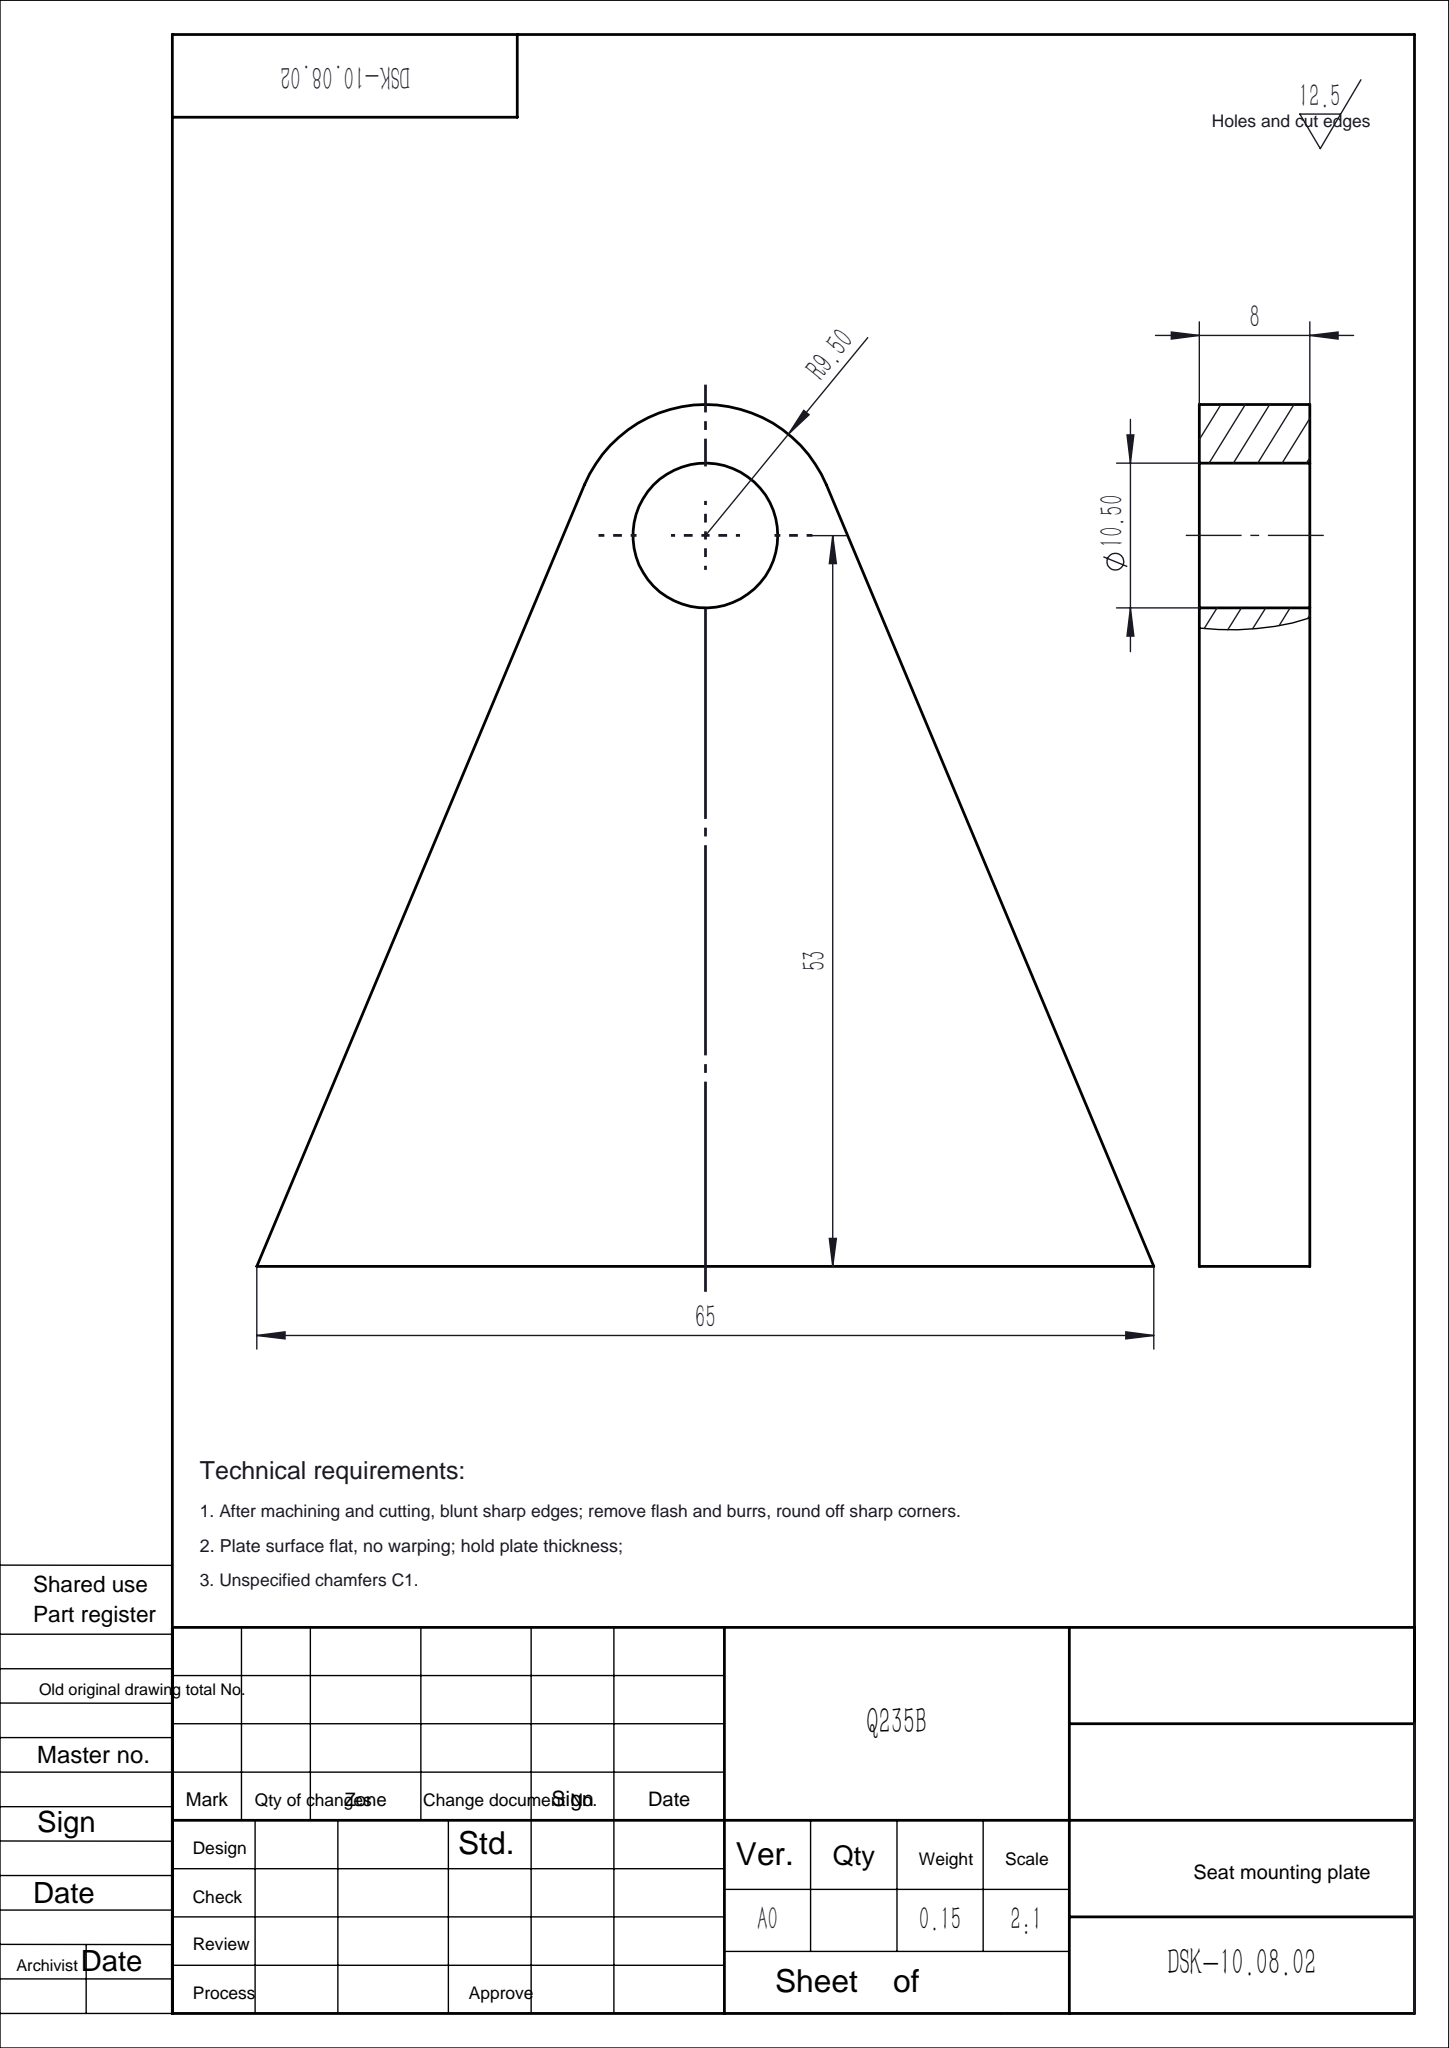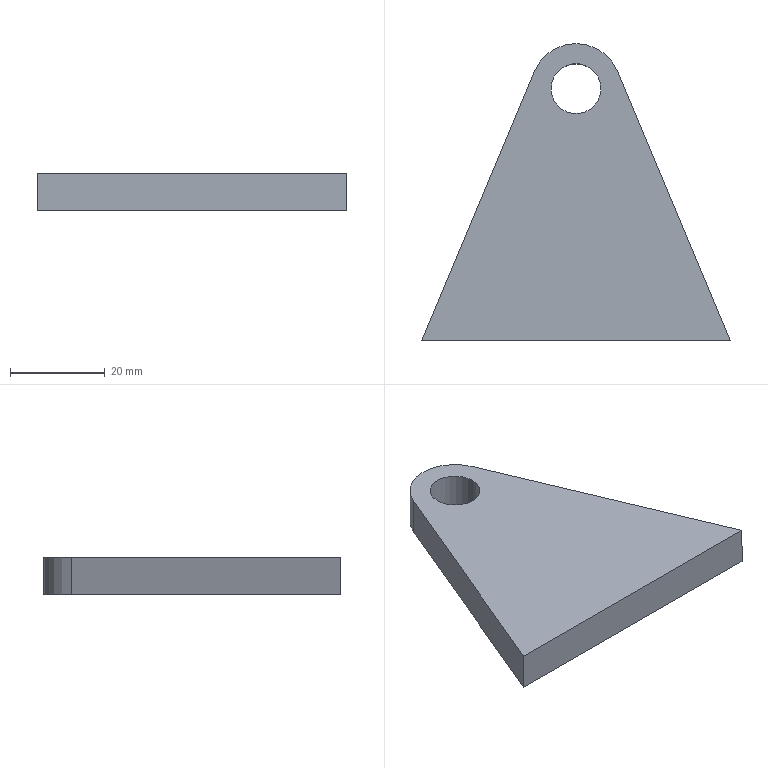Part | SolidWorks | features Extrusion 1 | 1 solid | 8 faces | box 65 x 62.5 x 8 mm | volume 18605 mm3 | plane 5 | cylinder 3 | commonest cylinder face diameters 10.5 x2 19 x1
STEP:
#1=CARTESIAN_POINT('',(-5.25,53.,8.));
#2=VERTEX_POINT('',#1);
#3=CARTESIAN_POINT('',(5.25,53.,8.));
#4=VERTEX_POINT('',#3);
#5=CARTESIAN_POINT('',(0.,53.,8.));
#6=DIRECTION('',(0.,0.,1.));
#7=DIRECTION('',(1.,0.,0.));
#8=AXIS2_PLACEMENT_3D('',#5,#6,#7);
#9=CIRCLE('',#8,5.25);
#10=EDGE_CURVE('',#2,#4,#9,.T.);
#11=ORIENTED_EDGE('',*,*,#10,.T.);
#12=CARTESIAN_POINT('',(5.25,53.,0.));
#13=VERTEX_POINT('',#12);
#14=CARTESIAN_POINT('',(5.25,53.,8.));
#15=DIRECTION('',(0.,0.,-1.));
#16=VECTOR('',#15,1000.);
#17=LINE('',#14,#16);
#18=EDGE_CURVE('',#4,#13,#17,.T.);
#19=ORIENTED_EDGE('',*,*,#18,.T.);
#20=CARTESIAN_POINT('',(-5.25,53.,0.));
#21=VERTEX_POINT('',#20);
#22=CARTESIAN_POINT('',(0.,53.,0.));
#23=DIRECTION('',(0.,0.,1.));
#24=DIRECTION('',(1.,0.,0.));
#25=AXIS2_PLACEMENT_3D('',#22,#23,#24);
#26=CIRCLE('',#25,5.25);
#27=EDGE_CURVE('',#21,#13,#26,.T.);
#28=ORIENTED_EDGE('',*,*,#27,.F.);
#29=CARTESIAN_POINT('',(-5.25,53.,8.));
#30=DIRECTION('',(0.,0.,-1.));
#31=VECTOR('',#30,1000.);
#32=LINE('',#29,#31);
#33=EDGE_CURVE('',#2,#21,#32,.T.);
#34=ORIENTED_EDGE('',*,*,#33,.F.);
#35=EDGE_LOOP('',(#11,#19,#28,#34));
#36=FACE_OUTER_BOUND('',#35,.T.);
#37=CARTESIAN_POINT('',(0.,53.,8.));
#38=DIRECTION('',(0.,0.,-1.));
#39=DIRECTION('',(-1.,0.,0.));
#40=AXIS2_PLACEMENT_3D('',#37,#38,#39);
#41=CYLINDRICAL_SURFACE('',#40,5.25);
#42=ADVANCED_FACE('',(#36),#41,.F.);
#43=CARTESIAN_POINT('',(32.5,0.,8.));
#44=VERTEX_POINT('',#43);
#45=CARTESIAN_POINT('',(8.762,56.67,8.));
#46=VERTEX_POINT('',#45);
#47=CARTESIAN_POINT('',(32.5,0.,8.));
#48=DIRECTION('',(-0.3863,0.9224,0.));
#49=VECTOR('',#48,1000.);
#50=LINE('',#47,#49);
#51=EDGE_CURVE('',#44,#46,#50,.T.);
#52=ORIENTED_EDGE('',*,*,#51,.T.);
#53=CARTESIAN_POINT('',(-8.762,56.67,8.));
#54=VERTEX_POINT('',#53);
#55=CARTESIAN_POINT('',(0.,53.,8.));
#56=DIRECTION('',(0.,0.,1.));
#57=DIRECTION('',(1.,0.,0.));
#58=AXIS2_PLACEMENT_3D('',#55,#56,#57);
#59=CIRCLE('',#58,9.5);
#60=EDGE_CURVE('',#46,#54,#59,.T.);
#61=ORIENTED_EDGE('',*,*,#60,.T.);
#62=CARTESIAN_POINT('',(-32.5,0.,8.));
#63=VERTEX_POINT('',#62);
#64=CARTESIAN_POINT('',(-32.5,0.,8.));
#65=DIRECTION('',(-0.3863,-0.9224,0.));
#66=VECTOR('',#65,1000.);
#67=LINE('',#64,#66);
#68=EDGE_CURVE('',#54,#63,#67,.T.);
#69=ORIENTED_EDGE('',*,*,#68,.T.);
#70=CARTESIAN_POINT('',(-32.5,0.,8.));
#71=DIRECTION('',(1.,0.,0.));
#72=VECTOR('',#71,1000.);
#73=LINE('',#70,#72);
#74=EDGE_CURVE('',#63,#44,#73,.T.);
#75=ORIENTED_EDGE('',*,*,#74,.T.);
#76=EDGE_LOOP('',(#52,#61,#69,#75));
#77=FACE_OUTER_BOUND('',#76,.T.);
#78=ORIENTED_EDGE('',*,*,#10,.F.);
#79=CARTESIAN_POINT('',(0.,53.,8.));
#80=DIRECTION('',(0.,0.,1.));
#81=DIRECTION('',(1.,0.,0.));
#82=AXIS2_PLACEMENT_3D('',#79,#80,#81);
#83=CIRCLE('',#82,5.25);
#84=EDGE_CURVE('',#4,#2,#83,.T.);
#85=ORIENTED_EDGE('',*,*,#84,.F.);
#86=EDGE_LOOP('',(#78,#85));
#87=FACE_BOUND('',#86,.T.);
#88=CARTESIAN_POINT('',(0.,53.,8.));
#89=DIRECTION('',(0.,0.,1.));
#90=DIRECTION('',(1.,0.,0.));
#91=AXIS2_PLACEMENT_3D('',#88,#89,#90);
#92=PLANE('',#91);
#93=ADVANCED_FACE('',(#77,#87),#92,.T.);
#94=CARTESIAN_POINT('',(32.5,0.,0.));
#95=VERTEX_POINT('',#94);
#96=CARTESIAN_POINT('',(8.762,56.67,0.));
#97=VERTEX_POINT('',#96);
#98=CARTESIAN_POINT('',(32.5,0.,0.));
#99=DIRECTION('',(-0.3863,0.9224,0.));
#100=VECTOR('',#99,1000.);
#101=LINE('',#98,#100);
#102=EDGE_CURVE('',#95,#97,#101,.T.);
#103=ORIENTED_EDGE('',*,*,#102,.F.);
#104=CARTESIAN_POINT('',(-32.5,0.,0.));
#105=VERTEX_POINT('',#104);
#106=CARTESIAN_POINT('',(-32.5,0.,0.));
#107=DIRECTION('',(1.,0.,0.));
#108=VECTOR('',#107,1000.);
#109=LINE('',#106,#108);
#110=EDGE_CURVE('',#105,#95,#109,.T.);
#111=ORIENTED_EDGE('',*,*,#110,.F.);
#112=CARTESIAN_POINT('',(-8.762,56.67,0.));
#113=VERTEX_POINT('',#112);
#114=CARTESIAN_POINT('',(-32.5,0.,0.));
#115=DIRECTION('',(-0.3863,-0.9224,0.));
#116=VECTOR('',#115,1000.);
#117=LINE('',#114,#116);
#118=EDGE_CURVE('',#113,#105,#117,.T.);
#119=ORIENTED_EDGE('',*,*,#118,.F.);
#120=CARTESIAN_POINT('',(0.,53.,0.));
#121=DIRECTION('',(0.,0.,1.));
#122=DIRECTION('',(1.,0.,0.));
#123=AXIS2_PLACEMENT_3D('',#120,#121,#122);
#124=CIRCLE('',#123,9.5);
#125=EDGE_CURVE('',#97,#113,#124,.T.);
#126=ORIENTED_EDGE('',*,*,#125,.F.);
#127=EDGE_LOOP('',(#103,#111,#119,#126));
#128=FACE_OUTER_BOUND('',#127,.T.);
#129=ORIENTED_EDGE('',*,*,#27,.T.);
#130=CARTESIAN_POINT('',(0.,53.,0.));
#131=DIRECTION('',(0.,0.,1.));
#132=DIRECTION('',(1.,0.,0.));
#133=AXIS2_PLACEMENT_3D('',#130,#131,#132);
#134=CIRCLE('',#133,5.25);
#135=EDGE_CURVE('',#13,#21,#134,.T.);
#136=ORIENTED_EDGE('',*,*,#135,.T.);
#137=EDGE_LOOP('',(#129,#136));
#138=FACE_BOUND('',#137,.T.);
#139=CARTESIAN_POINT('',(0.,53.,0.));
#140=DIRECTION('',(0.,0.,1.));
#141=DIRECTION('',(1.,0.,0.));
#142=AXIS2_PLACEMENT_3D('',#139,#140,#141);
#143=PLANE('',#142);
#144=ADVANCED_FACE('',(#128,#138),#143,.F.);
#145=ORIENTED_EDGE('',*,*,#102,.T.);
#146=CARTESIAN_POINT('',(8.762,56.67,8.));
#147=DIRECTION('',(0.,0.,-1.));
#148=VECTOR('',#147,1000.);
#149=LINE('',#146,#148);
#150=EDGE_CURVE('',#46,#97,#149,.T.);
#151=ORIENTED_EDGE('',*,*,#150,.F.);
#152=ORIENTED_EDGE('',*,*,#51,.F.);
#153=CARTESIAN_POINT('',(32.5,0.,8.));
#154=DIRECTION('',(0.,0.,-1.));
#155=VECTOR('',#154,1000.);
#156=LINE('',#153,#155);
#157=EDGE_CURVE('',#44,#95,#156,.T.);
#158=ORIENTED_EDGE('',*,*,#157,.T.);
#159=EDGE_LOOP('',(#145,#151,#152,#158));
#160=FACE_OUTER_BOUND('',#159,.T.);
#161=CARTESIAN_POINT('',(32.5,0.,8.));
#162=DIRECTION('',(-0.9224,-0.3863,0.));
#163=DIRECTION('',(0.3863,-0.9224,0.));
#164=AXIS2_PLACEMENT_3D('',#161,#162,#163);
#165=PLANE('',#164);
#166=ADVANCED_FACE('',(#160),#165,.F.);
#167=ORIENTED_EDGE('',*,*,#125,.T.);
#168=CARTESIAN_POINT('',(-8.762,56.67,8.));
#169=DIRECTION('',(0.,0.,-1.));
#170=VECTOR('',#169,1000.);
#171=LINE('',#168,#170);
#172=EDGE_CURVE('',#54,#113,#171,.T.);
#173=ORIENTED_EDGE('',*,*,#172,.F.);
#174=ORIENTED_EDGE('',*,*,#60,.F.);
#175=ORIENTED_EDGE('',*,*,#150,.T.);
#176=EDGE_LOOP('',(#167,#173,#174,#175));
#177=FACE_OUTER_BOUND('',#176,.T.);
#178=CARTESIAN_POINT('',(0.,53.,8.));
#179=DIRECTION('',(0.,0.,-1.));
#180=DIRECTION('',(-1.,0.,0.));
#181=AXIS2_PLACEMENT_3D('',#178,#179,#180);
#182=CYLINDRICAL_SURFACE('',#181,9.5);
#183=ADVANCED_FACE('',(#177),#182,.T.);
#184=ORIENTED_EDGE('',*,*,#118,.T.);
#185=CARTESIAN_POINT('',(-32.5,0.,8.));
#186=DIRECTION('',(0.,0.,-1.));
#187=VECTOR('',#186,1000.);
#188=LINE('',#185,#187);
#189=EDGE_CURVE('',#63,#105,#188,.T.);
#190=ORIENTED_EDGE('',*,*,#189,.F.);
#191=ORIENTED_EDGE('',*,*,#68,.F.);
#192=ORIENTED_EDGE('',*,*,#172,.T.);
#193=EDGE_LOOP('',(#184,#190,#191,#192));
#194=FACE_OUTER_BOUND('',#193,.T.);
#195=CARTESIAN_POINT('',(-32.5,0.,8.));
#196=DIRECTION('',(0.9224,-0.3863,0.));
#197=DIRECTION('',(0.3863,0.9224,0.));
#198=AXIS2_PLACEMENT_3D('',#195,#196,#197);
#199=PLANE('',#198);
#200=ADVANCED_FACE('',(#194),#199,.F.);
#201=ORIENTED_EDGE('',*,*,#110,.T.);
#202=ORIENTED_EDGE('',*,*,#157,.F.);
#203=ORIENTED_EDGE('',*,*,#74,.F.);
#204=ORIENTED_EDGE('',*,*,#189,.T.);
#205=EDGE_LOOP('',(#201,#202,#203,#204));
#206=FACE_OUTER_BOUND('',#205,.T.);
#207=CARTESIAN_POINT('',(-32.5,0.,8.));
#208=DIRECTION('',(0.,1.,0.));
#209=DIRECTION('',(-1.,0.,0.));
#210=AXIS2_PLACEMENT_3D('',#207,#208,#209);
#211=PLANE('',#210);
#212=ADVANCED_FACE('',(#206),#211,.F.);
#213=ORIENTED_EDGE('',*,*,#18,.F.);
#214=ORIENTED_EDGE('',*,*,#84,.T.);
#215=ORIENTED_EDGE('',*,*,#33,.T.);
#216=ORIENTED_EDGE('',*,*,#135,.F.);
#217=EDGE_LOOP('',(#213,#214,#215,#216));
#218=FACE_OUTER_BOUND('',#217,.T.);
#219=CARTESIAN_POINT('',(0.,53.,8.));
#220=DIRECTION('',(0.,0.,-1.));
#221=DIRECTION('',(-1.,0.,0.));
#222=AXIS2_PLACEMENT_3D('',#219,#220,#221);
#223=CYLINDRICAL_SURFACE('',#222,5.25);
#224=ADVANCED_FACE('',(#218),#223,.F.);
#225=CLOSED_SHELL('',(#42,#93,#144,#166,#183,#200,#212,#224));
#226=MANIFOLD_SOLID_BREP('',#225);
#227=CARTESIAN_POINT('',(0.,0.,0.));
#228=DIRECTION('',(0.,0.,1.));
#229=DIRECTION('',(1.,0.,0.));
#230=AXIS2_PLACEMENT_3D('',#227,#228,#229);
#231=(LENGTH_UNIT()NAMED_UNIT(*)SI_UNIT(.MILLI.,.METRE.));
#232=UNCERTAINTY_MEASURE_WITH_UNIT(LENGTH_MEASURE(0.00001),#231,'','');
#233=(NAMED_UNIT(*)PLANE_ANGLE_UNIT()SI_UNIT($,.RADIAN.));
#234=(NAMED_UNIT(*)SI_UNIT($,.STERADIAN.)SOLID_ANGLE_UNIT());
#235=(GEOMETRIC_REPRESENTATION_CONTEXT(3)GLOBAL_UNCERTAINTY_ASSIGNED_CONTEXT((#232))GLOBAL_UNIT_ASSIGNED_CONTEXT((#231,#233,#234))REPRESENTATION_CONTEXT('',''));
#236=ADVANCED_BREP_SHAPE_REPRESENTATION('',(#226,#230),#235);